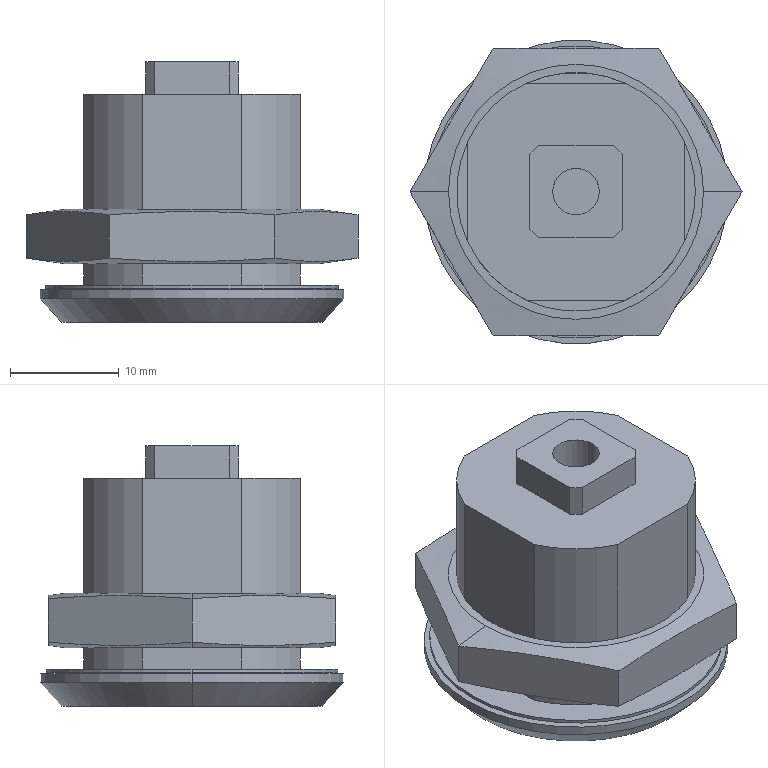Part | SolidWorks | features BaseBody 1 | 1 solid | 72 faces | box 30.6 x 28 x 24 mm | volume 9184 mm3 | plane 35 | cylinder 23 | cone 6 | sphere 5 | torus 3 | commonest cylinder face diameters 22 x13 4.3 x2 22.3 x2 25 x2 27 x2 28 x2